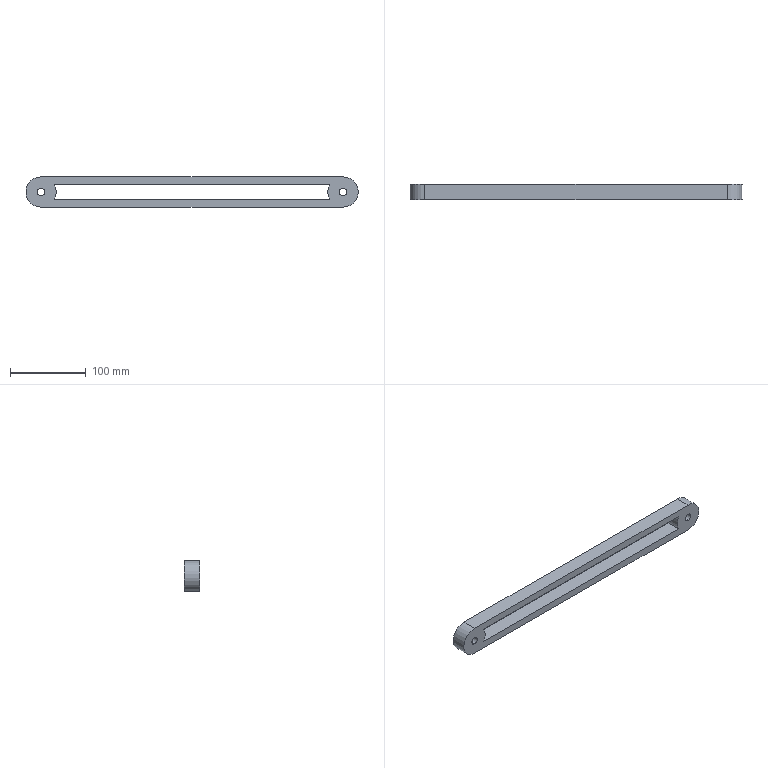Part | SolidWorks | features ICE 3, Extrusion 1 | 1 solid | 14 faces | box 440 x 20 x 40 mm | volume 197297 mm3 | cylinder 8 | plane 6 | commonest cylinder face diameters 10 x4 40 x4
STEP:
#1=CARTESIAN_POINT('',(200.,0.,-5.));
#2=VERTEX_POINT('',#1);
#3=CARTESIAN_POINT('',(200.,0.,5.));
#4=VERTEX_POINT('',#3);
#5=CARTESIAN_POINT('',(200.,0.,0.));
#6=DIRECTION('',(0.,1.,0.));
#7=DIRECTION('',(0.,0.,1.));
#8=AXIS2_PLACEMENT_3D('',#5,#6,#7);
#9=CIRCLE('',#8,5.);
#10=EDGE_CURVE('',#2,#4,#9,.T.);
#11=ORIENTED_EDGE('',*,*,#10,.F.);
#12=CARTESIAN_POINT('',(200.,20.,-5.));
#13=VERTEX_POINT('',#12);
#14=CARTESIAN_POINT('',(200.,0.,-5.));
#15=DIRECTION('',(0.,1.,0.));
#16=VECTOR('',#15,1000.);
#17=LINE('',#14,#16);
#18=EDGE_CURVE('',#2,#13,#17,.T.);
#19=ORIENTED_EDGE('',*,*,#18,.T.);
#20=CARTESIAN_POINT('',(200.,20.,5.));
#21=VERTEX_POINT('',#20);
#22=CARTESIAN_POINT('',(200.,20.,0.));
#23=DIRECTION('',(0.,1.,0.));
#24=DIRECTION('',(0.,0.,1.));
#25=AXIS2_PLACEMENT_3D('',#22,#23,#24);
#26=CIRCLE('',#25,5.);
#27=EDGE_CURVE('',#13,#21,#26,.T.);
#28=ORIENTED_EDGE('',*,*,#27,.T.);
#29=CARTESIAN_POINT('',(200.,0.,5.));
#30=DIRECTION('',(0.,1.,0.));
#31=VECTOR('',#30,1000.);
#32=LINE('',#29,#31);
#33=EDGE_CURVE('',#4,#21,#32,.T.);
#34=ORIENTED_EDGE('',*,*,#33,.F.);
#35=EDGE_LOOP('',(#11,#19,#28,#34));
#36=FACE_OUTER_BOUND('',#35,.T.);
#37=CARTESIAN_POINT('',(200.,0.,0.));
#38=DIRECTION('',(0.,1.,0.));
#39=DIRECTION('',(0.,0.,1.));
#40=AXIS2_PLACEMENT_3D('',#37,#38,#39);
#41=CYLINDRICAL_SURFACE('',#40,5.);
#42=ADVANCED_FACE('',(#36),#41,.F.);
#43=CARTESIAN_POINT('',(-200.,0.,-5.));
#44=VERTEX_POINT('',#43);
#45=CARTESIAN_POINT('',(-200.,0.,5.));
#46=VERTEX_POINT('',#45);
#47=CARTESIAN_POINT('',(-200.,0.,0.));
#48=DIRECTION('',(0.,1.,0.));
#49=DIRECTION('',(0.,0.,-1.));
#50=AXIS2_PLACEMENT_3D('',#47,#48,#49);
#51=CIRCLE('',#50,5.);
#52=EDGE_CURVE('',#44,#46,#51,.T.);
#53=ORIENTED_EDGE('',*,*,#52,.F.);
#54=CARTESIAN_POINT('',(-200.,20.,-5.));
#55=VERTEX_POINT('',#54);
#56=CARTESIAN_POINT('',(-200.,0.,-5.));
#57=DIRECTION('',(0.,1.,0.));
#58=VECTOR('',#57,1000.);
#59=LINE('',#56,#58);
#60=EDGE_CURVE('',#44,#55,#59,.T.);
#61=ORIENTED_EDGE('',*,*,#60,.T.);
#62=CARTESIAN_POINT('',(-200.,20.,5.));
#63=VERTEX_POINT('',#62);
#64=CARTESIAN_POINT('',(-200.,20.,0.));
#65=DIRECTION('',(0.,1.,0.));
#66=DIRECTION('',(0.,0.,-1.));
#67=AXIS2_PLACEMENT_3D('',#64,#65,#66);
#68=CIRCLE('',#67,5.);
#69=EDGE_CURVE('',#55,#63,#68,.T.);
#70=ORIENTED_EDGE('',*,*,#69,.T.);
#71=CARTESIAN_POINT('',(-200.,0.,5.));
#72=DIRECTION('',(0.,1.,0.));
#73=VECTOR('',#72,1000.);
#74=LINE('',#71,#73);
#75=EDGE_CURVE('',#46,#63,#74,.T.);
#76=ORIENTED_EDGE('',*,*,#75,.F.);
#77=EDGE_LOOP('',(#53,#61,#70,#76));
#78=FACE_OUTER_BOUND('',#77,.T.);
#79=CARTESIAN_POINT('',(-200.,0.,0.));
#80=DIRECTION('',(0.,1.,0.));
#81=DIRECTION('',(0.,0.,1.));
#82=AXIS2_PLACEMENT_3D('',#79,#80,#81);
#83=CYLINDRICAL_SURFACE('',#82,5.);
#84=ADVANCED_FACE('',(#78),#83,.F.);
#85=CARTESIAN_POINT('',(200.,0.,-20.));
#86=VERTEX_POINT('',#85);
#87=CARTESIAN_POINT('',(-200.,0.,-20.));
#88=VERTEX_POINT('',#87);
#89=CARTESIAN_POINT('',(-200.,0.,-20.));
#90=DIRECTION('',(-1.,0.,0.));
#91=VECTOR('',#90,1000.);
#92=LINE('',#89,#91);
#93=EDGE_CURVE('',#86,#88,#92,.T.);
#94=ORIENTED_EDGE('',*,*,#93,.T.);
#95=CARTESIAN_POINT('',(-200.,20.,-20.));
#96=VERTEX_POINT('',#95);
#97=CARTESIAN_POINT('',(-200.,20.,-20.));
#98=DIRECTION('',(0.,-1.,0.));
#99=VECTOR('',#98,1000.);
#100=LINE('',#97,#99);
#101=EDGE_CURVE('',#96,#88,#100,.T.);
#102=ORIENTED_EDGE('',*,*,#101,.F.);
#103=CARTESIAN_POINT('',(200.,20.,-20.));
#104=VERTEX_POINT('',#103);
#105=CARTESIAN_POINT('',(-200.,20.,-20.));
#106=DIRECTION('',(-1.,0.,0.));
#107=VECTOR('',#106,1000.);
#108=LINE('',#105,#107);
#109=EDGE_CURVE('',#104,#96,#108,.T.);
#110=ORIENTED_EDGE('',*,*,#109,.F.);
#111=CARTESIAN_POINT('',(200.,20.,-20.));
#112=DIRECTION('',(0.,-1.,0.));
#113=VECTOR('',#112,1000.);
#114=LINE('',#111,#113);
#115=EDGE_CURVE('',#104,#86,#114,.T.);
#116=ORIENTED_EDGE('',*,*,#115,.T.);
#117=EDGE_LOOP('',(#94,#102,#110,#116));
#118=FACE_OUTER_BOUND('',#117,.T.);
#119=CARTESIAN_POINT('',(-200.,20.,-20.));
#120=DIRECTION('',(0.,0.,1.));
#121=DIRECTION('',(1.,0.,0.));
#122=AXIS2_PLACEMENT_3D('',#119,#120,#121);
#123=PLANE('',#122);
#124=ADVANCED_FACE('',(#118),#123,.F.);
#125=CARTESIAN_POINT('',(-200.,0.,20.));
#126=VERTEX_POINT('',#125);
#127=CARTESIAN_POINT('',(200.,0.,20.));
#128=VERTEX_POINT('',#127);
#129=CARTESIAN_POINT('',(-200.,0.,20.));
#130=DIRECTION('',(1.,0.,0.));
#131=VECTOR('',#130,1000.);
#132=LINE('',#129,#131);
#133=EDGE_CURVE('',#126,#128,#132,.T.);
#134=ORIENTED_EDGE('',*,*,#133,.T.);
#135=CARTESIAN_POINT('',(200.,20.,20.));
#136=VERTEX_POINT('',#135);
#137=CARTESIAN_POINT('',(200.,20.,20.));
#138=DIRECTION('',(0.,-1.,0.));
#139=VECTOR('',#138,1000.);
#140=LINE('',#137,#139);
#141=EDGE_CURVE('',#136,#128,#140,.T.);
#142=ORIENTED_EDGE('',*,*,#141,.F.);
#143=CARTESIAN_POINT('',(-200.,20.,20.));
#144=VERTEX_POINT('',#143);
#145=CARTESIAN_POINT('',(-200.,20.,20.));
#146=DIRECTION('',(1.,0.,0.));
#147=VECTOR('',#146,1000.);
#148=LINE('',#145,#147);
#149=EDGE_CURVE('',#144,#136,#148,.T.);
#150=ORIENTED_EDGE('',*,*,#149,.F.);
#151=CARTESIAN_POINT('',(-200.,20.,20.));
#152=DIRECTION('',(0.,-1.,0.));
#153=VECTOR('',#152,1000.);
#154=LINE('',#151,#153);
#155=EDGE_CURVE('',#144,#126,#154,.T.);
#156=ORIENTED_EDGE('',*,*,#155,.T.);
#157=EDGE_LOOP('',(#134,#142,#150,#156));
#158=FACE_OUTER_BOUND('',#157,.T.);
#159=CARTESIAN_POINT('',(-200.,20.,20.));
#160=DIRECTION('',(0.,0.,-1.));
#161=DIRECTION('',(-1.,0.,0.));
#162=AXIS2_PLACEMENT_3D('',#159,#160,#161);
#163=PLANE('',#162);
#164=ADVANCED_FACE('',(#158),#163,.F.);
#165=CARTESIAN_POINT('',(200.,20.,0.));
#166=DIRECTION('',(0.,1.,0.));
#167=DIRECTION('',(0.,0.,1.));
#168=AXIS2_PLACEMENT_3D('',#165,#166,#167);
#169=CIRCLE('',#168,5.);
#170=EDGE_CURVE('',#21,#13,#169,.T.);
#171=ORIENTED_EDGE('',*,*,#170,.F.);
#172=ORIENTED_EDGE('',*,*,#27,.F.);
#173=EDGE_LOOP('',(#171,#172));
#174=FACE_BOUND('',#173,.T.);
#175=CARTESIAN_POINT('',(-200.,20.,0.));
#176=DIRECTION('',(0.,1.,0.));
#177=DIRECTION('',(0.,0.,-1.));
#178=AXIS2_PLACEMENT_3D('',#175,#176,#177);
#179=CIRCLE('',#178,5.);
#180=EDGE_CURVE('',#63,#55,#179,.T.);
#181=ORIENTED_EDGE('',*,*,#180,.F.);
#182=ORIENTED_EDGE('',*,*,#69,.F.);
#183=EDGE_LOOP('',(#181,#182));
#184=FACE_BOUND('',#183,.T.);
#185=CARTESIAN_POINT('',(-182.679,20.,10.));
#186=VERTEX_POINT('',#185);
#187=CARTESIAN_POINT('',(182.679,20.,10.));
#188=VERTEX_POINT('',#187);
#189=CARTESIAN_POINT('',(-190.,20.,10.));
#190=DIRECTION('',(1.,0.,0.));
#191=VECTOR('',#190,1000.);
#192=LINE('',#189,#191);
#193=EDGE_CURVE('',#186,#188,#192,.T.);
#194=ORIENTED_EDGE('',*,*,#193,.F.);
#195=CARTESIAN_POINT('',(-182.679,20.,-10.));
#196=VERTEX_POINT('',#195);
#197=CARTESIAN_POINT('',(-200.,20.,0.));
#198=DIRECTION('',(0.,1.,0.));
#199=DIRECTION('',(0.,0.,-1.));
#200=AXIS2_PLACEMENT_3D('',#197,#198,#199);
#201=CIRCLE('',#200,20.);
#202=EDGE_CURVE('',#186,#196,#201,.T.);
#203=ORIENTED_EDGE('',*,*,#202,.T.);
#204=CARTESIAN_POINT('',(182.679,20.,-10.));
#205=VERTEX_POINT('',#204);
#206=CARTESIAN_POINT('',(190.,20.,-10.));
#207=DIRECTION('',(-1.,0.,0.));
#208=VECTOR('',#207,1000.);
#209=LINE('',#206,#208);
#210=EDGE_CURVE('',#205,#196,#209,.T.);
#211=ORIENTED_EDGE('',*,*,#210,.F.);
#212=CARTESIAN_POINT('',(200.,20.,0.));
#213=DIRECTION('',(0.,1.,0.));
#214=DIRECTION('',(0.,0.,1.));
#215=AXIS2_PLACEMENT_3D('',#212,#213,#214);
#216=CIRCLE('',#215,20.);
#217=EDGE_CURVE('',#205,#188,#216,.T.);
#218=ORIENTED_EDGE('',*,*,#217,.T.);
#219=EDGE_LOOP('',(#194,#203,#211,#218));
#220=FACE_BOUND('',#219,.T.);
#221=ORIENTED_EDGE('',*,*,#109,.T.);
#222=CARTESIAN_POINT('',(-200.,20.,0.));
#223=DIRECTION('',(0.,1.,0.));
#224=DIRECTION('',(0.,0.,-1.));
#225=AXIS2_PLACEMENT_3D('',#222,#223,#224);
#226=CIRCLE('',#225,20.);
#227=EDGE_CURVE('',#96,#144,#226,.T.);
#228=ORIENTED_EDGE('',*,*,#227,.T.);
#229=ORIENTED_EDGE('',*,*,#149,.T.);
#230=CARTESIAN_POINT('',(200.,20.,0.));
#231=DIRECTION('',(0.,1.,0.));
#232=DIRECTION('',(0.,0.,1.));
#233=AXIS2_PLACEMENT_3D('',#230,#231,#232);
#234=CIRCLE('',#233,20.);
#235=EDGE_CURVE('',#136,#104,#234,.T.);
#236=ORIENTED_EDGE('',*,*,#235,.T.);
#237=EDGE_LOOP('',(#221,#228,#229,#236));
#238=FACE_OUTER_BOUND('',#237,.T.);
#239=CARTESIAN_POINT('',(0.,20.,0.));
#240=DIRECTION('',(0.,1.,0.));
#241=DIRECTION('',(0.,0.,1.));
#242=AXIS2_PLACEMENT_3D('',#239,#240,#241);
#243=PLANE('',#242);
#244=ADVANCED_FACE('',(#174,#184,#220,#238),#243,.T.);
#245=CARTESIAN_POINT('',(200.,0.,0.));
#246=DIRECTION('',(0.,1.,0.));
#247=DIRECTION('',(0.,0.,1.));
#248=AXIS2_PLACEMENT_3D('',#245,#246,#247);
#249=CIRCLE('',#248,5.);
#250=EDGE_CURVE('',#4,#2,#249,.T.);
#251=ORIENTED_EDGE('',*,*,#250,.T.);
#252=ORIENTED_EDGE('',*,*,#10,.T.);
#253=EDGE_LOOP('',(#251,#252));
#254=FACE_BOUND('',#253,.T.);
#255=CARTESIAN_POINT('',(-200.,0.,0.));
#256=DIRECTION('',(0.,1.,0.));
#257=DIRECTION('',(0.,0.,-1.));
#258=AXIS2_PLACEMENT_3D('',#255,#256,#257);
#259=CIRCLE('',#258,5.);
#260=EDGE_CURVE('',#46,#44,#259,.T.);
#261=ORIENTED_EDGE('',*,*,#260,.T.);
#262=ORIENTED_EDGE('',*,*,#52,.T.);
#263=EDGE_LOOP('',(#261,#262));
#264=FACE_BOUND('',#263,.T.);
#265=CARTESIAN_POINT('',(-182.679,0.,10.));
#266=VERTEX_POINT('',#265);
#267=CARTESIAN_POINT('',(-182.679,0.,-10.));
#268=VERTEX_POINT('',#267);
#269=CARTESIAN_POINT('',(-200.,0.,0.));
#270=DIRECTION('',(0.,1.,0.));
#271=DIRECTION('',(0.,0.,-1.));
#272=AXIS2_PLACEMENT_3D('',#269,#270,#271);
#273=CIRCLE('',#272,20.);
#274=EDGE_CURVE('',#266,#268,#273,.T.);
#275=ORIENTED_EDGE('',*,*,#274,.F.);
#276=CARTESIAN_POINT('',(182.679,0.,10.));
#277=VERTEX_POINT('',#276);
#278=CARTESIAN_POINT('',(-190.,0.,10.));
#279=DIRECTION('',(1.,0.,0.));
#280=VECTOR('',#279,1000.);
#281=LINE('',#278,#280);
#282=EDGE_CURVE('',#266,#277,#281,.T.);
#283=ORIENTED_EDGE('',*,*,#282,.T.);
#284=CARTESIAN_POINT('',(182.679,0.,-10.));
#285=VERTEX_POINT('',#284);
#286=CARTESIAN_POINT('',(200.,0.,0.));
#287=DIRECTION('',(0.,1.,0.));
#288=DIRECTION('',(0.,0.,1.));
#289=AXIS2_PLACEMENT_3D('',#286,#287,#288);
#290=CIRCLE('',#289,20.);
#291=EDGE_CURVE('',#285,#277,#290,.T.);
#292=ORIENTED_EDGE('',*,*,#291,.F.);
#293=CARTESIAN_POINT('',(190.,0.,-10.));
#294=DIRECTION('',(-1.,0.,0.));
#295=VECTOR('',#294,1000.);
#296=LINE('',#293,#295);
#297=EDGE_CURVE('',#285,#268,#296,.T.);
#298=ORIENTED_EDGE('',*,*,#297,.T.);
#299=EDGE_LOOP('',(#275,#283,#292,#298));
#300=FACE_BOUND('',#299,.T.);
#301=ORIENTED_EDGE('',*,*,#133,.F.);
#302=CARTESIAN_POINT('',(-200.,0.,0.));
#303=DIRECTION('',(0.,1.,0.));
#304=DIRECTION('',(0.,0.,-1.));
#305=AXIS2_PLACEMENT_3D('',#302,#303,#304);
#306=CIRCLE('',#305,20.);
#307=EDGE_CURVE('',#88,#126,#306,.T.);
#308=ORIENTED_EDGE('',*,*,#307,.F.);
#309=ORIENTED_EDGE('',*,*,#93,.F.);
#310=CARTESIAN_POINT('',(200.,0.,0.));
#311=DIRECTION('',(0.,1.,0.));
#312=DIRECTION('',(0.,0.,1.));
#313=AXIS2_PLACEMENT_3D('',#310,#311,#312);
#314=CIRCLE('',#313,20.);
#315=EDGE_CURVE('',#128,#86,#314,.T.);
#316=ORIENTED_EDGE('',*,*,#315,.F.);
#317=EDGE_LOOP('',(#301,#308,#309,#316));
#318=FACE_OUTER_BOUND('',#317,.T.);
#319=CARTESIAN_POINT('',(0.,0.,0.));
#320=DIRECTION('',(0.,1.,0.));
#321=DIRECTION('',(0.,0.,1.));
#322=AXIS2_PLACEMENT_3D('',#319,#320,#321);
#323=PLANE('',#322);
#324=ADVANCED_FACE('',(#254,#264,#300,#318),#323,.F.);
#325=ORIENTED_EDGE('',*,*,#282,.F.);
#326=CARTESIAN_POINT('',(-182.679,0.,10.));
#327=DIRECTION('',(0.,1.,0.));
#328=VECTOR('',#327,1000.);
#329=LINE('',#326,#328);
#330=EDGE_CURVE('',#266,#186,#329,.T.);
#331=ORIENTED_EDGE('',*,*,#330,.T.);
#332=ORIENTED_EDGE('',*,*,#193,.T.);
#333=CARTESIAN_POINT('',(182.679,0.,10.));
#334=DIRECTION('',(0.,-1.,0.));
#335=VECTOR('',#334,1000.);
#336=LINE('',#333,#335);
#337=EDGE_CURVE('',#188,#277,#336,.T.);
#338=ORIENTED_EDGE('',*,*,#337,.T.);
#339=EDGE_LOOP('',(#325,#331,#332,#338));
#340=FACE_OUTER_BOUND('',#339,.T.);
#341=CARTESIAN_POINT('',(-190.,0.,10.));
#342=DIRECTION('',(0.,0.,1.));
#343=DIRECTION('',(1.,0.,0.));
#344=AXIS2_PLACEMENT_3D('',#341,#342,#343);
#345=PLANE('',#344);
#346=ADVANCED_FACE('',(#340),#345,.F.);
#347=ORIENTED_EDGE('',*,*,#210,.T.);
#348=CARTESIAN_POINT('',(-182.679,0.,-10.));
#349=DIRECTION('',(0.,-1.,0.));
#350=VECTOR('',#349,1000.);
#351=LINE('',#348,#350);
#352=EDGE_CURVE('',#196,#268,#351,.T.);
#353=ORIENTED_EDGE('',*,*,#352,.T.);
#354=ORIENTED_EDGE('',*,*,#297,.F.);
#355=CARTESIAN_POINT('',(182.679,0.,-10.));
#356=DIRECTION('',(0.,1.,0.));
#357=VECTOR('',#356,1000.);
#358=LINE('',#355,#357);
#359=EDGE_CURVE('',#285,#205,#358,.T.);
#360=ORIENTED_EDGE('',*,*,#359,.T.);
#361=EDGE_LOOP('',(#347,#353,#354,#360));
#362=FACE_OUTER_BOUND('',#361,.T.);
#363=CARTESIAN_POINT('',(190.,0.,-10.));
#364=DIRECTION('',(0.,0.,-1.));
#365=DIRECTION('',(-1.,0.,0.));
#366=AXIS2_PLACEMENT_3D('',#363,#364,#365);
#367=PLANE('',#366);
#368=ADVANCED_FACE('',(#362),#367,.F.);
#369=ORIENTED_EDGE('',*,*,#337,.F.);
#370=ORIENTED_EDGE('',*,*,#217,.F.);
#371=ORIENTED_EDGE('',*,*,#359,.F.);
#372=ORIENTED_EDGE('',*,*,#291,.T.);
#373=EDGE_LOOP('',(#369,#370,#371,#372));
#374=FACE_OUTER_BOUND('',#373,.T.);
#375=CARTESIAN_POINT('',(200.,0.,0.));
#376=DIRECTION('',(0.,1.,0.));
#377=DIRECTION('',(0.,0.,1.));
#378=AXIS2_PLACEMENT_3D('',#375,#376,#377);
#379=CYLINDRICAL_SURFACE('',#378,20.);
#380=ADVANCED_FACE('',(#374),#379,.T.);
#381=ORIENTED_EDGE('',*,*,#315,.T.);
#382=ORIENTED_EDGE('',*,*,#115,.F.);
#383=ORIENTED_EDGE('',*,*,#235,.F.);
#384=ORIENTED_EDGE('',*,*,#141,.T.);
#385=EDGE_LOOP('',(#381,#382,#383,#384));
#386=FACE_OUTER_BOUND('',#385,.T.);
#387=CARTESIAN_POINT('',(200.,0.,0.));
#388=DIRECTION('',(0.,1.,0.));
#389=DIRECTION('',(0.,0.,1.));
#390=AXIS2_PLACEMENT_3D('',#387,#388,#389);
#391=CYLINDRICAL_SURFACE('',#390,20.);
#392=ADVANCED_FACE('',(#386),#391,.T.);
#393=ORIENTED_EDGE('',*,*,#330,.F.);
#394=ORIENTED_EDGE('',*,*,#274,.T.);
#395=ORIENTED_EDGE('',*,*,#352,.F.);
#396=ORIENTED_EDGE('',*,*,#202,.F.);
#397=EDGE_LOOP('',(#393,#394,#395,#396));
#398=FACE_OUTER_BOUND('',#397,.T.);
#399=CARTESIAN_POINT('',(-200.,0.,0.));
#400=DIRECTION('',(0.,1.,0.));
#401=DIRECTION('',(0.,0.,1.));
#402=AXIS2_PLACEMENT_3D('',#399,#400,#401);
#403=CYLINDRICAL_SURFACE('',#402,20.);
#404=ADVANCED_FACE('',(#398),#403,.T.);
#405=ORIENTED_EDGE('',*,*,#101,.T.);
#406=ORIENTED_EDGE('',*,*,#307,.T.);
#407=ORIENTED_EDGE('',*,*,#155,.F.);
#408=ORIENTED_EDGE('',*,*,#227,.F.);
#409=EDGE_LOOP('',(#405,#406,#407,#408));
#410=FACE_OUTER_BOUND('',#409,.T.);
#411=CARTESIAN_POINT('',(-200.,0.,0.));
#412=DIRECTION('',(0.,1.,0.));
#413=DIRECTION('',(0.,0.,1.));
#414=AXIS2_PLACEMENT_3D('',#411,#412,#413);
#415=CYLINDRICAL_SURFACE('',#414,20.);
#416=ADVANCED_FACE('',(#410),#415,.T.);
#417=ORIENTED_EDGE('',*,*,#60,.F.);
#418=ORIENTED_EDGE('',*,*,#260,.F.);
#419=ORIENTED_EDGE('',*,*,#75,.T.);
#420=ORIENTED_EDGE('',*,*,#180,.T.);
#421=EDGE_LOOP('',(#417,#418,#419,#420));
#422=FACE_OUTER_BOUND('',#421,.T.);
#423=CARTESIAN_POINT('',(-200.,0.,0.));
#424=DIRECTION('',(0.,1.,0.));
#425=DIRECTION('',(0.,0.,1.));
#426=AXIS2_PLACEMENT_3D('',#423,#424,#425);
#427=CYLINDRICAL_SURFACE('',#426,5.);
#428=ADVANCED_FACE('',(#422),#427,.F.);
#429=ORIENTED_EDGE('',*,*,#18,.F.);
#430=ORIENTED_EDGE('',*,*,#250,.F.);
#431=ORIENTED_EDGE('',*,*,#33,.T.);
#432=ORIENTED_EDGE('',*,*,#170,.T.);
#433=EDGE_LOOP('',(#429,#430,#431,#432));
#434=FACE_OUTER_BOUND('',#433,.T.);
#435=CARTESIAN_POINT('',(200.,0.,0.));
#436=DIRECTION('',(0.,1.,0.));
#437=DIRECTION('',(0.,0.,1.));
#438=AXIS2_PLACEMENT_3D('',#435,#436,#437);
#439=CYLINDRICAL_SURFACE('',#438,5.);
#440=ADVANCED_FACE('',(#434),#439,.F.);
#441=CLOSED_SHELL('',(#42,#84,#124,#164,#244,#324,#346,#368,#380,#392,#404,#416,#428,#440));
#442=MANIFOLD_SOLID_BREP('',#441);
#443=CARTESIAN_POINT('',(0.,0.,0.));
#444=DIRECTION('',(0.,0.,1.));
#445=DIRECTION('',(1.,0.,0.));
#446=AXIS2_PLACEMENT_3D('',#443,#444,#445);
#447=(LENGTH_UNIT()NAMED_UNIT(*)SI_UNIT(.MILLI.,.METRE.));
#448=UNCERTAINTY_MEASURE_WITH_UNIT(LENGTH_MEASURE(0.00001),#447,'','');
#449=(NAMED_UNIT(*)PLANE_ANGLE_UNIT()SI_UNIT($,.RADIAN.));
#450=(NAMED_UNIT(*)SI_UNIT($,.STERADIAN.)SOLID_ANGLE_UNIT());
#451=(GEOMETRIC_REPRESENTATION_CONTEXT(3)GLOBAL_UNCERTAINTY_ASSIGNED_CONTEXT((#448))GLOBAL_UNIT_ASSIGNED_CONTEXT((#447,#449,#450))REPRESENTATION_CONTEXT('',''));
#452=ADVANCED_BREP_SHAPE_REPRESENTATION('',(#442,#446),#451);